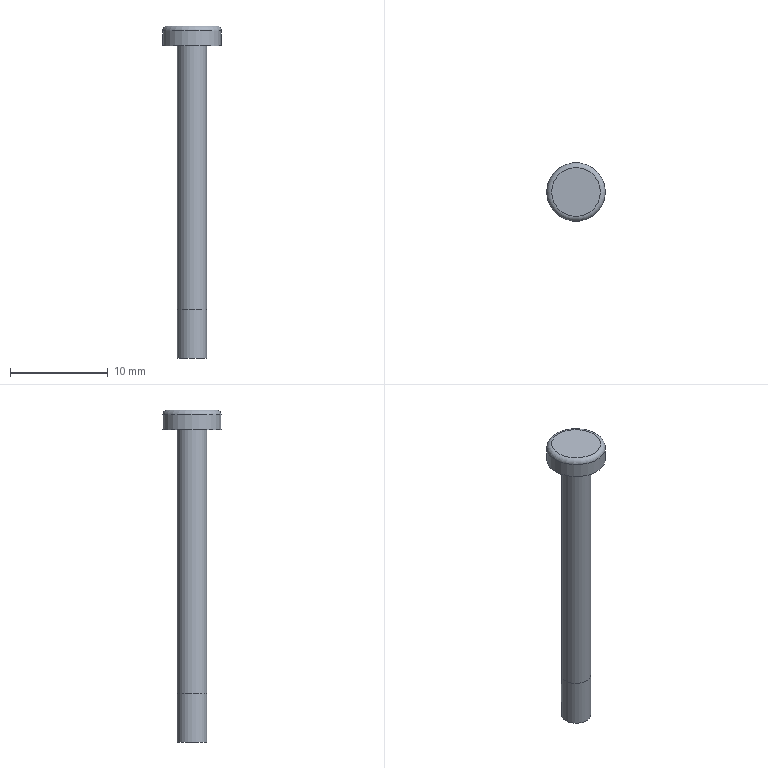Part | STEP file | 1-54.4 | 1 solid | 7 faces | box 6 x 6 x 34 mm | volume 281.77 mm3 | plane 3 | cylinder 3 | torus 1 | commonest cylinder face diameters 3 x2 6 x1
STEP:
#1=CARTESIAN_POINT('',(0.,0.,0.));
#2=DIRECTION('',(0.,0.,1.));
#3=DIRECTION('',(1.,0.,0.));
#4=AXIS2_PLACEMENT_3D('',#1,#2,#3);
#5=CARTESIAN_POINT('',(3.,0.,0.));
#6=VERTEX_POINT('',#5);
#7=CARTESIAN_POINT('',(0.,0.,0.));
#8=DIRECTION('',(0.,0.,1.));
#9=DIRECTION('',(1.,0.,0.));
#10=AXIS2_PLACEMENT_3D('',#7,#8,#9);
#11=CIRCLE('',#10,3.);
#12=CARTESIAN_POINT('',(-0.8038,0.,0.));
#13=DIRECTION('',(0.,0.,1.));
#14=DIRECTION('',(1.,0.,0.));
#15=AXIS2_PLACEMENT_3D('',#12,#13,#14);
#16=PLANE('',#15);
#17=CARTESIAN_POINT('',(0.8038,0.));
#18=DIRECTION('',(1.,0.));
#19=AXIS2_PLACEMENT_2D('',#17,#18);
#20=CIRCLE('',#19,3.);
#21=(GEOMETRIC_REPRESENTATION_CONTEXT(2)PARAMETRIC_REPRESENTATION_CONTEXT()REPRESENTATION_CONTEXT('',''));
#22=DEFINITIONAL_REPRESENTATION('',(#20),#21);
#23=PCURVE('',#16,#22);
#24=CARTESIAN_POINT('',(0.,0.,0.));
#25=DIRECTION('',(0.,0.,1.));
#26=DIRECTION('',(1.,0.,0.));
#27=AXIS2_PLACEMENT_3D('',#24,#25,#26);
#28=CYLINDRICAL_SURFACE('',#27,3.);
#29=CARTESIAN_POINT('',(0.,0.));
#30=DIRECTION('',(1.,0.));
#31=VECTOR('',#30,1.);
#32=LINE('',#29,#31);
#33=(GEOMETRIC_REPRESENTATION_CONTEXT(2)PARAMETRIC_REPRESENTATION_CONTEXT()REPRESENTATION_CONTEXT('',''));
#34=DEFINITIONAL_REPRESENTATION('',(#32),#33);
#35=PCURVE('',#28,#34);
#36=SURFACE_CURVE('',#11,(#23,#35),.PCURVE_S1.);
#37=EDGE_CURVE('',#6,#6,#36,.T.);
#38=ORIENTED_EDGE('',*,*,#37,.T.);
#39=EDGE_LOOP('',(#38));
#40=FACE_BOUND('',#39,.F.);
#41=CARTESIAN_POINT('',(1.5,0.,0.));
#42=VERTEX_POINT('',#41);
#43=CARTESIAN_POINT('',(0.,0.,0.));
#44=DIRECTION('',(0.,0.,1.));
#45=DIRECTION('',(1.,0.,0.));
#46=AXIS2_PLACEMENT_3D('',#43,#44,#45);
#47=CIRCLE('',#46,1.5);
#48=CARTESIAN_POINT('',(0.8038,0.));
#49=DIRECTION('',(1.,0.));
#50=AXIS2_PLACEMENT_2D('',#48,#49);
#51=CIRCLE('',#50,1.5);
#52=(GEOMETRIC_REPRESENTATION_CONTEXT(2)PARAMETRIC_REPRESENTATION_CONTEXT()REPRESENTATION_CONTEXT('',''));
#53=DEFINITIONAL_REPRESENTATION('',(#51),#52);
#54=PCURVE('',#16,#53);
#55=CARTESIAN_POINT('',(0.,0.,0.));
#56=DIRECTION('',(0.,0.,-1.));
#57=DIRECTION('',(1.,0.,0.));
#58=AXIS2_PLACEMENT_3D('',#55,#56,#57);
#59=CYLINDRICAL_SURFACE('',#58,1.5);
#60=CARTESIAN_POINT('',(6.283,0.));
#61=DIRECTION('',(-1.,0.));
#62=VECTOR('',#61,1.);
#63=LINE('',#60,#62);
#64=(GEOMETRIC_REPRESENTATION_CONTEXT(2)PARAMETRIC_REPRESENTATION_CONTEXT()REPRESENTATION_CONTEXT('',''));
#65=DEFINITIONAL_REPRESENTATION('',(#63),#64);
#66=PCURVE('',#59,#65);
#67=SURFACE_CURVE('',#47,(#54,#66),.PCURVE_S1.);
#68=EDGE_CURVE('',#42,#42,#67,.T.);
#69=ORIENTED_EDGE('',*,*,#68,.F.);
#70=EDGE_LOOP('',(#69));
#71=FACE_BOUND('',#70,.F.);
#72=ADVANCED_FACE('',(#40,#71),#16,.F.);
#73=CARTESIAN_POINT('',(1.5,0.,-32.));
#74=VERTEX_POINT('',#73);
#75=CARTESIAN_POINT('',(0.,0.,-32.));
#76=DIRECTION('',(0.,0.,1.));
#77=DIRECTION('',(1.,0.,0.));
#78=AXIS2_PLACEMENT_3D('',#75,#76,#77);
#79=CIRCLE('',#78,1.5);
#80=CARTESIAN_POINT('',(-0.4019,0.,-32.));
#81=DIRECTION('',(0.,0.,1.));
#82=DIRECTION('',(1.,0.,0.));
#83=AXIS2_PLACEMENT_3D('',#80,#81,#82);
#84=PLANE('',#83);
#85=CARTESIAN_POINT('',(0.4019,0.));
#86=DIRECTION('',(1.,0.));
#87=AXIS2_PLACEMENT_2D('',#85,#86);
#88=CIRCLE('',#87,1.5);
#89=(GEOMETRIC_REPRESENTATION_CONTEXT(2)PARAMETRIC_REPRESENTATION_CONTEXT()REPRESENTATION_CONTEXT('',''));
#90=DEFINITIONAL_REPRESENTATION('',(#88),#89);
#91=PCURVE('',#84,#90);
#92=CARTESIAN_POINT('',(0.,0.,-27.));
#93=DIRECTION('',(0.,0.,-1.));
#94=DIRECTION('',(1.,0.,0.));
#95=AXIS2_PLACEMENT_3D('',#92,#93,#94);
#96=CYLINDRICAL_SURFACE('',#95,1.5);
#97=CARTESIAN_POINT('',(6.283,5.));
#98=DIRECTION('',(-1.,0.));
#99=VECTOR('',#98,1.);
#100=LINE('',#97,#99);
#101=(GEOMETRIC_REPRESENTATION_CONTEXT(2)PARAMETRIC_REPRESENTATION_CONTEXT()REPRESENTATION_CONTEXT('',''));
#102=DEFINITIONAL_REPRESENTATION('',(#100),#101);
#103=PCURVE('',#96,#102);
#104=SURFACE_CURVE('',#79,(#91,#103),.PCURVE_S1.);
#105=EDGE_CURVE('',#74,#74,#104,.T.);
#106=ORIENTED_EDGE('',*,*,#105,.T.);
#107=EDGE_LOOP('',(#106));
#108=FACE_BOUND('',#107,.F.);
#109=ADVANCED_FACE('',(#108),#84,.F.);
#110=CARTESIAN_POINT('',(2.5,0.,2.));
#111=VERTEX_POINT('',#110);
#112=CARTESIAN_POINT('',(0.,0.,2.));
#113=DIRECTION('',(0.,0.,-1.));
#114=DIRECTION('',(1.,0.,0.));
#115=AXIS2_PLACEMENT_3D('',#112,#113,#114);
#116=CIRCLE('',#115,2.5);
#117=CARTESIAN_POINT('',(-0.8038,0.,2.));
#118=DIRECTION('',(0.,0.,1.));
#119=DIRECTION('',(1.,0.,0.));
#120=AXIS2_PLACEMENT_3D('',#117,#118,#119);
#121=PLANE('',#120);
#122=CARTESIAN_POINT('',(3.304,0.));
#123=CARTESIAN_POINT('',(3.304,-4.33));
#124=CARTESIAN_POINT('',(-0.4462,-2.165));
#125=CARTESIAN_POINT('',(-4.196,0.));
#126=CARTESIAN_POINT('',(-0.4462,2.165));
#127=CARTESIAN_POINT('',(3.304,4.33));
#128=CARTESIAN_POINT('',(3.304,0.));
#129=(BOUNDED_CURVE()B_SPLINE_CURVE(2,(#122,#123,#124,#125,#126,#127,#128),.UNSPECIFIED.,.T.,.F.)B_SPLINE_CURVE_WITH_KNOTS((1,2,2,2,2,1),(-2.094,0.,2.094,4.189,6.283,8.378),.UNSPECIFIED.)CURVE()GEOMETRIC_REPRESENTATION_ITEM()RATIONAL_B_SPLINE_CURVE((1.,0.5,1.,0.5,1.,0.5,1.))REPRESENTATION_ITEM(''));
#130=(GEOMETRIC_REPRESENTATION_CONTEXT(2)PARAMETRIC_REPRESENTATION_CONTEXT()REPRESENTATION_CONTEXT('',''));
#131=DEFINITIONAL_REPRESENTATION('',(#129),#130);
#132=PCURVE('',#121,#131);
#133=CARTESIAN_POINT('',(0.,0.,1.5));
#134=DIRECTION('',(0.,0.,1.));
#135=DIRECTION('',(1.,0.,0.));
#136=AXIS2_PLACEMENT_3D('',#133,#134,#135);
#137=TOROIDAL_SURFACE('',#136,2.5,0.5);
#138=CARTESIAN_POINT('',(6.283,1.571));
#139=DIRECTION('',(-1.,0.));
#140=VECTOR('',#139,1.);
#141=LINE('',#138,#140);
#142=(GEOMETRIC_REPRESENTATION_CONTEXT(2)PARAMETRIC_REPRESENTATION_CONTEXT()REPRESENTATION_CONTEXT('',''));
#143=DEFINITIONAL_REPRESENTATION('',(#141),#142);
#144=PCURVE('',#137,#143);
#145=SURFACE_CURVE('',#116,(#132,#144),.PCURVE_S1.);
#146=EDGE_CURVE('',#111,#111,#145,.T.);
#147=ORIENTED_EDGE('',*,*,#146,.F.);
#148=EDGE_LOOP('',(#147));
#149=FACE_BOUND('',#148,.T.);
#150=ADVANCED_FACE('',(#149),#121,.T.);
#151=ORIENTED_EDGE('',*,*,#37,.T.);
#152=CARTESIAN_POINT('',(3.,0.,1.5));
#153=VERTEX_POINT('',#152);
#154=CARTESIAN_POINT('',(3.,0.,0.));
#155=DIRECTION('',(0.,0.,1.));
#156=VECTOR('',#155,1.);
#157=LINE('',#154,#156);
#158=CARTESIAN_POINT('',(6.283,0.));
#159=DIRECTION('',(0.,1.));
#160=VECTOR('',#159,1.);
#161=LINE('',#158,#160);
#162=(GEOMETRIC_REPRESENTATION_CONTEXT(2)PARAMETRIC_REPRESENTATION_CONTEXT()REPRESENTATION_CONTEXT('',''));
#163=DEFINITIONAL_REPRESENTATION('',(#161),#162);
#164=PCURVE('',#28,#163);
#165=CARTESIAN_POINT('',(0.,0.));
#166=DIRECTION('',(0.,1.));
#167=VECTOR('',#166,1.);
#168=LINE('',#165,#167);
#169=(GEOMETRIC_REPRESENTATION_CONTEXT(2)PARAMETRIC_REPRESENTATION_CONTEXT()REPRESENTATION_CONTEXT('',''));
#170=DEFINITIONAL_REPRESENTATION('',(#168),#169);
#171=PCURVE('',#28,#170);
#172=SEAM_CURVE('',#157,(#164,#171),.PCURVE_S1.);
#173=EDGE_CURVE('',#6,#153,#172,.T.);
#174=ORIENTED_EDGE('',*,*,#173,.T.);
#175=CARTESIAN_POINT('',(0.,0.,1.5));
#176=DIRECTION('',(0.,0.,-1.));
#177=DIRECTION('',(1.,0.,0.));
#178=AXIS2_PLACEMENT_3D('',#175,#176,#177);
#179=CIRCLE('',#178,3.);
#180=CARTESIAN_POINT('',(6.283,1.5));
#181=DIRECTION('',(-1.,0.));
#182=VECTOR('',#181,1.);
#183=LINE('',#180,#182);
#184=(GEOMETRIC_REPRESENTATION_CONTEXT(2)PARAMETRIC_REPRESENTATION_CONTEXT()REPRESENTATION_CONTEXT('',''));
#185=DEFINITIONAL_REPRESENTATION('',(#183),#184);
#186=PCURVE('',#28,#185);
#187=CARTESIAN_POINT('',(6.283,0.));
#188=DIRECTION('',(-1.,0.));
#189=VECTOR('',#188,1.);
#190=LINE('',#187,#189);
#191=(GEOMETRIC_REPRESENTATION_CONTEXT(2)PARAMETRIC_REPRESENTATION_CONTEXT()REPRESENTATION_CONTEXT('',''));
#192=DEFINITIONAL_REPRESENTATION('',(#190),#191);
#193=PCURVE('',#137,#192);
#194=SURFACE_CURVE('',#179,(#186,#193),.PCURVE_S1.);
#195=EDGE_CURVE('',#153,#153,#194,.T.);
#196=ORIENTED_EDGE('',*,*,#195,.T.);
#197=ORIENTED_EDGE('',*,*,#173,.F.);
#198=EDGE_LOOP('',(#151,#174,#196,#197));
#199=FACE_BOUND('',#198,.T.);
#200=ADVANCED_FACE('',(#199),#28,.T.);
#201=CARTESIAN_POINT('',(2.5,0.,1.5));
#202=DIRECTION('',(0.,1.,0.));
#203=DIRECTION('',(0.,0.,1.));
#204=AXIS2_PLACEMENT_3D('',#201,#202,#203);
#205=CIRCLE('',#204,0.5);
#206=CARTESIAN_POINT('',(0.,1.571));
#207=CARTESIAN_POINT('',(0.,1.547));
#208=CARTESIAN_POINT('',(0.,1.499));
#209=CARTESIAN_POINT('',(0.,1.428));
#210=CARTESIAN_POINT('',(0.,1.357));
#211=CARTESIAN_POINT('',(0.,1.285));
#212=CARTESIAN_POINT('',(0.,1.214));
#213=CARTESIAN_POINT('',(0.,1.142));
#214=CARTESIAN_POINT('',(0.,1.071));
#215=CARTESIAN_POINT('',(0.,0.9996));
#216=CARTESIAN_POINT('',(0.,0.9282));
#217=CARTESIAN_POINT('',(0.,0.8568));
#218=CARTESIAN_POINT('',(0.,0.7854));
#219=CARTESIAN_POINT('',(0.,0.714));
#220=CARTESIAN_POINT('',(0.,0.6426));
#221=CARTESIAN_POINT('',(0.,0.5712));
#222=CARTESIAN_POINT('',(0.,0.4998));
#223=CARTESIAN_POINT('',(0.,0.4284));
#224=CARTESIAN_POINT('',(0.,0.357));
#225=CARTESIAN_POINT('',(0.,0.2856));
#226=CARTESIAN_POINT('',(0.,0.2142));
#227=CARTESIAN_POINT('',(0.,0.1428));
#228=CARTESIAN_POINT('',(0.,0.0714));
#229=CARTESIAN_POINT('',(0.,0.0238));
#230=CARTESIAN_POINT('',(0.,0.));
#231=B_SPLINE_CURVE_WITH_KNOTS('',3,(#206,#207,#208,#209,#210,#211,#212,#213,#214,#215,#216,#217,#218,#219,#220,#221,#222,#223,#224,#225,#226,#227,#228,#229,#230),.UNSPECIFIED.,.F.,.F.,(4,1,1,1,1,1,1,1,1,1,1,1,1,1,1,1,1,1,1,1,1,1,4),(0.,0.0714,0.1428,0.2142,0.2856,0.357,0.4284,0.4998,0.5712,0.6426,0.714,0.7854,0.8568,0.9282,0.9996,1.071,1.142,1.214,1.285,1.357,1.428,1.499,1.571),.QUASI_UNIFORM_KNOTS.);
#232=(GEOMETRIC_REPRESENTATION_CONTEXT(2)PARAMETRIC_REPRESENTATION_CONTEXT()REPRESENTATION_CONTEXT('',''));
#233=DEFINITIONAL_REPRESENTATION('',(#231),#232);
#234=PCURVE('',#137,#233);
#235=CARTESIAN_POINT('',(6.283,1.571));
#236=CARTESIAN_POINT('',(6.283,1.547));
#237=CARTESIAN_POINT('',(6.283,1.499));
#238=CARTESIAN_POINT('',(6.283,1.428));
#239=CARTESIAN_POINT('',(6.283,1.357));
#240=CARTESIAN_POINT('',(6.283,1.285));
#241=CARTESIAN_POINT('',(6.283,1.214));
#242=CARTESIAN_POINT('',(6.283,1.142));
#243=CARTESIAN_POINT('',(6.283,1.071));
#244=CARTESIAN_POINT('',(6.283,0.9996));
#245=CARTESIAN_POINT('',(6.283,0.9282));
#246=CARTESIAN_POINT('',(6.283,0.8568));
#247=CARTESIAN_POINT('',(6.283,0.7854));
#248=CARTESIAN_POINT('',(6.283,0.714));
#249=CARTESIAN_POINT('',(6.283,0.6426));
#250=CARTESIAN_POINT('',(6.283,0.5712));
#251=CARTESIAN_POINT('',(6.283,0.4998));
#252=CARTESIAN_POINT('',(6.283,0.4284));
#253=CARTESIAN_POINT('',(6.283,0.357));
#254=CARTESIAN_POINT('',(6.283,0.2856));
#255=CARTESIAN_POINT('',(6.283,0.2142));
#256=CARTESIAN_POINT('',(6.283,0.1428));
#257=CARTESIAN_POINT('',(6.283,0.0714));
#258=CARTESIAN_POINT('',(6.283,0.0238));
#259=CARTESIAN_POINT('',(6.283,0.));
#260=B_SPLINE_CURVE_WITH_KNOTS('',3,(#235,#236,#237,#238,#239,#240,#241,#242,#243,#244,#245,#246,#247,#248,#249,#250,#251,#252,#253,#254,#255,#256,#257,#258,#259),.UNSPECIFIED.,.F.,.F.,(4,1,1,1,1,1,1,1,1,1,1,1,1,1,1,1,1,1,1,1,1,1,4),(0.,0.0714,0.1428,0.2142,0.2856,0.357,0.4284,0.4998,0.5712,0.6426,0.714,0.7854,0.8568,0.9282,0.9996,1.071,1.142,1.214,1.285,1.357,1.428,1.499,1.571),.QUASI_UNIFORM_KNOTS.);
#261=(GEOMETRIC_REPRESENTATION_CONTEXT(2)PARAMETRIC_REPRESENTATION_CONTEXT()REPRESENTATION_CONTEXT('',''));
#262=DEFINITIONAL_REPRESENTATION('',(#260),#261);
#263=PCURVE('',#137,#262);
#264=SEAM_CURVE('',#205,(#234,#263),.PCURVE_S1.);
#265=EDGE_CURVE('',#111,#153,#264,.T.);
#266=ORIENTED_EDGE('',*,*,#265,.T.);
#267=ORIENTED_EDGE('',*,*,#195,.F.);
#268=ORIENTED_EDGE('',*,*,#265,.F.);
#269=ORIENTED_EDGE('',*,*,#146,.T.);
#270=EDGE_LOOP('',(#266,#267,#268,#269));
#271=FACE_BOUND('',#270,.T.);
#272=ADVANCED_FACE('',(#271),#137,.T.);
#273=CARTESIAN_POINT('',(1.5,0.,-27.));
#274=VERTEX_POINT('',#273);
#275=CARTESIAN_POINT('',(1.5,0.,0.));
#276=DIRECTION('',(0.,0.,-1.));
#277=VECTOR('',#276,1.);
#278=LINE('',#275,#277);
#279=CARTESIAN_POINT('',(6.283,0.));
#280=DIRECTION('',(0.,1.));
#281=VECTOR('',#280,1.);
#282=LINE('',#279,#281);
#283=(GEOMETRIC_REPRESENTATION_CONTEXT(2)PARAMETRIC_REPRESENTATION_CONTEXT()REPRESENTATION_CONTEXT('',''));
#284=DEFINITIONAL_REPRESENTATION('',(#282),#283);
#285=PCURVE('',#59,#284);
#286=CARTESIAN_POINT('',(0.,0.));
#287=DIRECTION('',(0.,1.));
#288=VECTOR('',#287,1.);
#289=LINE('',#286,#288);
#290=(GEOMETRIC_REPRESENTATION_CONTEXT(2)PARAMETRIC_REPRESENTATION_CONTEXT()REPRESENTATION_CONTEXT('',''));
#291=DEFINITIONAL_REPRESENTATION('',(#289),#290);
#292=PCURVE('',#59,#291);
#293=SEAM_CURVE('',#278,(#285,#292),.PCURVE_S1.);
#294=EDGE_CURVE('',#42,#274,#293,.T.);
#295=ORIENTED_EDGE('',*,*,#294,.T.);
#296=CARTESIAN_POINT('',(0.,0.,-27.));
#297=DIRECTION('',(0.,0.,1.));
#298=DIRECTION('',(1.,0.,0.));
#299=AXIS2_PLACEMENT_3D('',#296,#297,#298);
#300=CIRCLE('',#299,1.5);
#301=CARTESIAN_POINT('',(6.283,27.));
#302=DIRECTION('',(-1.,0.));
#303=VECTOR('',#302,1.);
#304=LINE('',#301,#303);
#305=(GEOMETRIC_REPRESENTATION_CONTEXT(2)PARAMETRIC_REPRESENTATION_CONTEXT()REPRESENTATION_CONTEXT('',''));
#306=DEFINITIONAL_REPRESENTATION('',(#304),#305);
#307=PCURVE('',#59,#306);
#308=CARTESIAN_POINT('',(6.283,0.));
#309=DIRECTION('',(-1.,0.));
#310=VECTOR('',#309,1.);
#311=LINE('',#308,#310);
#312=(GEOMETRIC_REPRESENTATION_CONTEXT(2)PARAMETRIC_REPRESENTATION_CONTEXT()REPRESENTATION_CONTEXT('',''));
#313=DEFINITIONAL_REPRESENTATION('',(#311),#312);
#314=PCURVE('',#96,#313);
#315=SURFACE_CURVE('',#300,(#307,#314),.PCURVE_S1.);
#316=EDGE_CURVE('',#274,#274,#315,.T.);
#317=ORIENTED_EDGE('',*,*,#316,.T.);
#318=ORIENTED_EDGE('',*,*,#294,.F.);
#319=ORIENTED_EDGE('',*,*,#68,.F.);
#320=EDGE_LOOP('',(#295,#317,#318,#319));
#321=FACE_BOUND('',#320,.T.);
#322=ADVANCED_FACE('',(#321),#59,.T.);
#323=CARTESIAN_POINT('',(1.5,0.,-27.));
#324=DIRECTION('',(0.,0.,-1.));
#325=VECTOR('',#324,1.);
#326=LINE('',#323,#325);
#327=CARTESIAN_POINT('',(0.,0.));
#328=DIRECTION('',(0.,1.));
#329=VECTOR('',#328,1.);
#330=LINE('',#327,#329);
#331=(GEOMETRIC_REPRESENTATION_CONTEXT(2)PARAMETRIC_REPRESENTATION_CONTEXT()REPRESENTATION_CONTEXT('',''));
#332=DEFINITIONAL_REPRESENTATION('',(#330),#331);
#333=PCURVE('',#96,#332);
#334=CARTESIAN_POINT('',(6.283,0.));
#335=DIRECTION('',(0.,1.));
#336=VECTOR('',#335,1.);
#337=LINE('',#334,#336);
#338=(GEOMETRIC_REPRESENTATION_CONTEXT(2)PARAMETRIC_REPRESENTATION_CONTEXT()REPRESENTATION_CONTEXT('',''));
#339=DEFINITIONAL_REPRESENTATION('',(#337),#338);
#340=PCURVE('',#96,#339);
#341=SEAM_CURVE('',#326,(#333,#340),.PCURVE_S1.);
#342=EDGE_CURVE('',#274,#74,#341,.T.);
#343=ORIENTED_EDGE('',*,*,#342,.F.);
#344=ORIENTED_EDGE('',*,*,#316,.F.);
#345=ORIENTED_EDGE('',*,*,#342,.T.);
#346=ORIENTED_EDGE('',*,*,#105,.T.);
#347=EDGE_LOOP('',(#343,#344,#345,#346));
#348=FACE_BOUND('',#347,.T.);
#349=ADVANCED_FACE('',(#348),#96,.T.);
#350=CLOSED_SHELL('',(#72,#109,#150,#200,#272,#322,#349));
#351=MANIFOLD_SOLID_BREP('',#350);
#352=(LENGTH_UNIT()NAMED_UNIT(*)SI_UNIT(.MILLI.,.METRE.));
#353=UNCERTAINTY_MEASURE_WITH_UNIT(LENGTH_MEASURE(0.0000001),#352,'','');
#354=(NAMED_UNIT(*)PLANE_ANGLE_UNIT()SI_UNIT($,.RADIAN.));
#355=(NAMED_UNIT(*)SI_UNIT($,.STERADIAN.)SOLID_ANGLE_UNIT());
#356=(GEOMETRIC_REPRESENTATION_CONTEXT(3)GLOBAL_UNCERTAINTY_ASSIGNED_CONTEXT((#353))GLOBAL_UNIT_ASSIGNED_CONTEXT((#352,#354,#355))REPRESENTATION_CONTEXT('',''));
#357=ADVANCED_BREP_SHAPE_REPRESENTATION('',(#4,#351),#356);